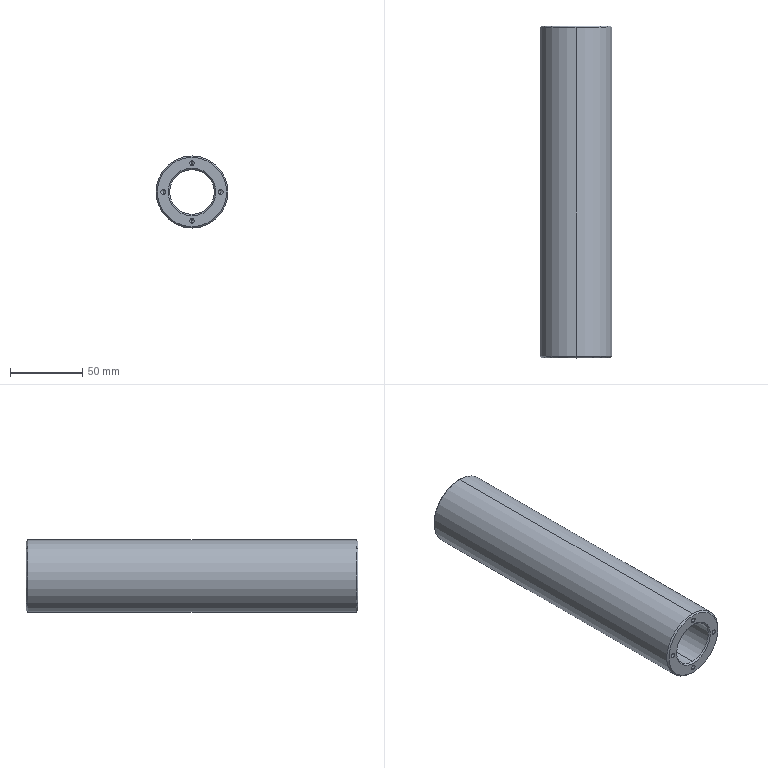Part | STEP file | 0229_212_Holder | 1 solid | 46 faces | box 50 x 230 x 50 mm | volume 276670 mm3 | cone 24 | cylinder 20 | plane 2 | commonest cylinder face diameters 3.3 x16 31 x2 50 x2